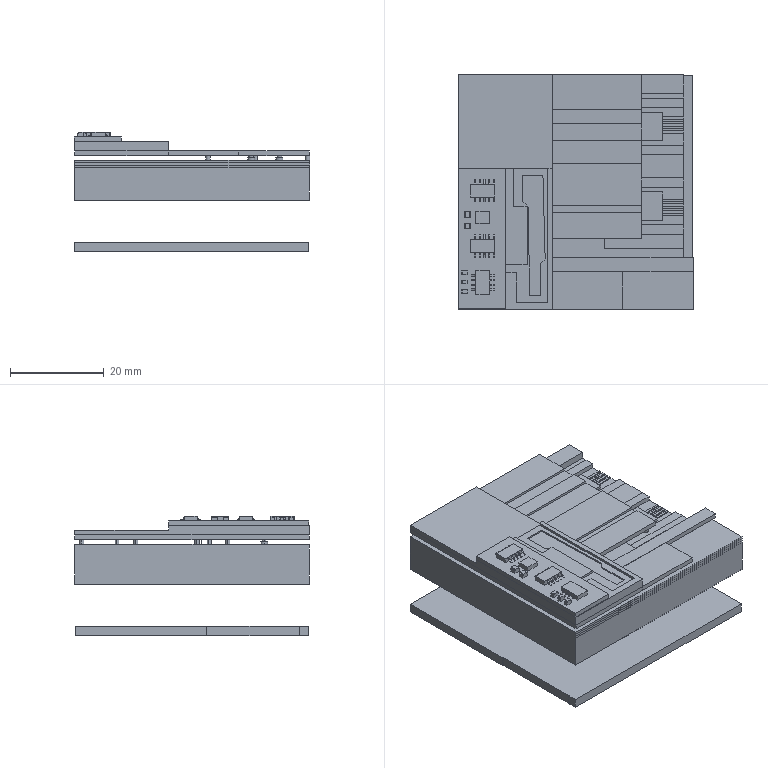Part | SolidWorks | features ICE 50, MoveCopyBody 5, LPattern 4, Split 3, Extrusion 1 | 63 solids | 566 faces | box 50.25 x 50 x 25.5 mm | volume 28187 mm3 | plane 534 | cylinder 32 | commonest cylinder face diameters 1 x26 1.5 x4 0.22 x2